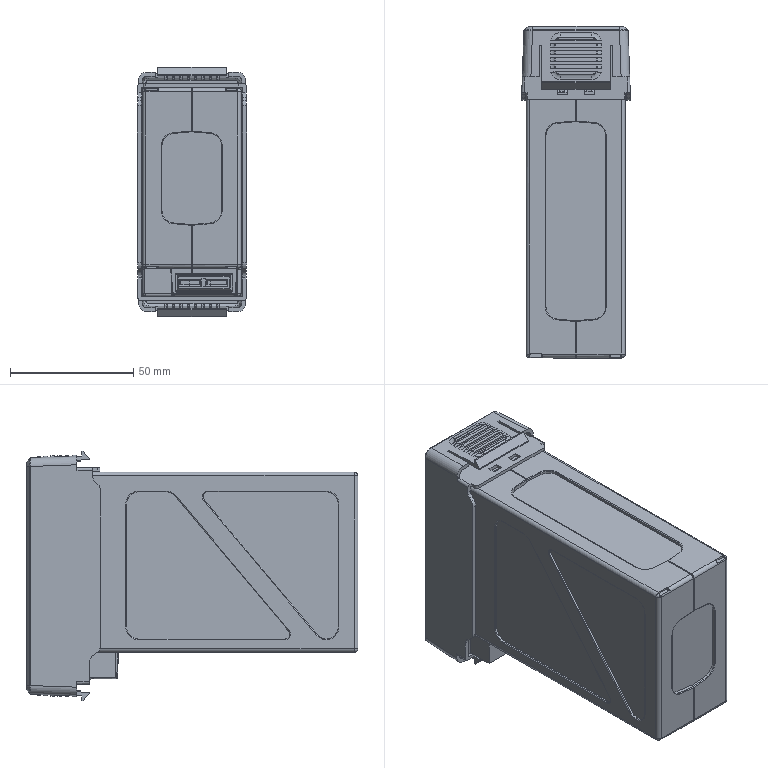Part | SolidWorks | features BaseBody 9, CenterOfMass 1 | 9 solids | 1591 faces | box 44.3 x 134.791 x 101.5 mm | volume 420051 mm3 | plane 1024 | cylinder 379 | spline 94 | torus 59 | cone 23 | sphere 12 | commonest cylinder face diameters 1 x103 0.6 x66 2 x39 3 x28 10 x22 4 x20